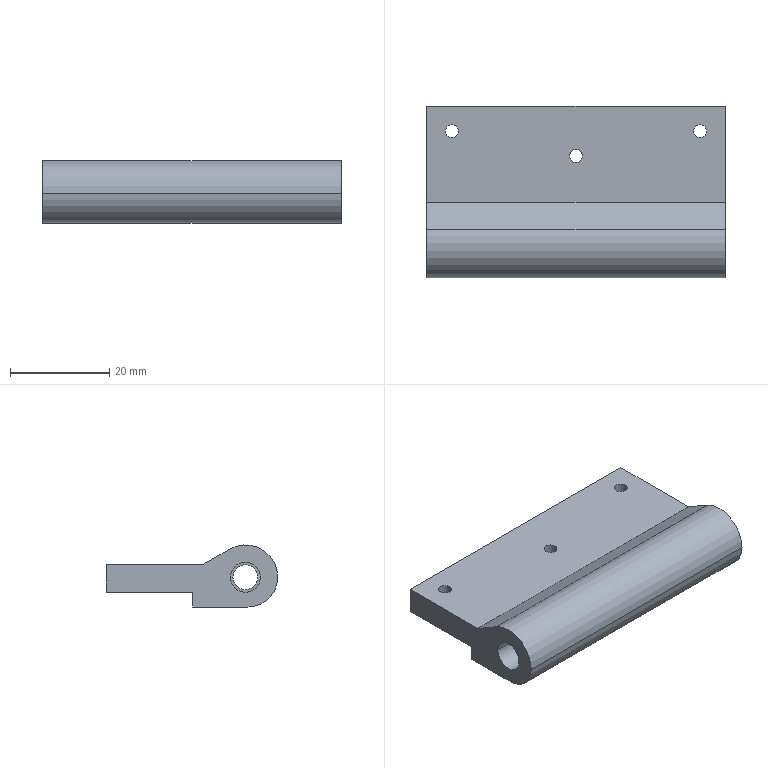NC program | NX | posted with a generic post | part box 60 x 34.5 x 12.5 mm
Whole program:
N10 G17 G21 G94 G90
(FACE_MILLING , TOOL : D63)
N12 T01 M6
N14 G54
N16 G17 G0 G90 X-97.5 Y20.5 B0. C0. S6500 M3
N18 G43 Z42.5 H1
N20 Z17.167
N22 G94 G1 Z14.167 F1250.
N24 X-66.
N26 X31.5
N28 Y-20.5
N30 X-66.
N32 X-97.5
N34 Z17.167
N36 G0 Z42.5
N38 Y20.5
N40 Z16.333
N42 G1 Z13.333
N44 X-66.
N46 X31.5
N48 Y-20.5
N50 X-66.
N52 X-97.5
N54 Z16.333
N56 G0 Z42.5
N58 Y20.5
N60 Z15.5
N62 G1 Z12.5
N64 X-66.
N66 X31.5
N68 Y-20.5
N70 X-66.
N72 X-97.5
N74 Z15.5
N76 G0 Z42.5
N78 M5
(FLOOR_WALL_2 , TOOL : D10)
N80 T10 M6
N82 G54
N84 G17 G0 G90 X-0.003 Y38. B0. C0. S9500 M3
N86 G43 Z42.5 H10
N88 Z14.525
N90 G94 G1 Z11.525 F2000.
N92 Y35.
N94 Y-35.
N96 X-4.786
N98 Y35.
N100 X-9.57
N102 Y-35.
N104 X-14.353
N106 Y35.
N108 Y38.
N110 Z14.525
N112 G0 Z42.5
N114 X-0.003
N116 Z13.55
N118 G1 Z10.55
N120 Y35.
N122 Y-35.
N124 X-4.786
N126 Y35.
N128 X-9.57
N130 Y-35.
N132 X-14.353
N134 Y35.
N136 Y38.
N138 Z13.55
N140 G0 Z42.5
N142 X-0.003
N144 Z12.575
N146 G1 Z9.575
N148 Y35.
N150 Y-35.
N152 X-4.786
N154 Y35.
N156 X-9.57
N158 Y-35.
N160 X-14.353
N162 Y35.
N164 Y38.15
N166 Z12.575
N168 G0 Z42.5
N170 X-0.003 Y38.
N172 Z11.6
N174 G1 Z8.6
N176 Y35.
N178 Y-35.
N180 X-4.786
N182 Y35.
N184 X-9.57
N186 Y-35.
N188 X-14.353
N190 Y35.
N192 Y38.15
N194 Z11.6
N196 G0 Z42.5
N198 M5
(FLOOR_WALL_1_COPY , TOOL : D10JING)
N200 T11 M6
N202 G54
N204 G17 G0 G90 X-0.001 Y38. B0. C0. S9500 M3
N206 G43 Z42.5 H11
N208 Z11.5
N210 G94 G1 Z8.5 F1250.
N212 Y35.
N214 Y-35.
N216 X-4.611
N218 Y35.
N220 X-9.22
N222 Y-35.
N224 X-13.83
N226 Y35.
N228 Y38.
N230 Z11.5
N232 G0 Z42.5
N234 X-14.33
N236 Z11.5
N238 G1 Z8.5
N240 Y35.
N242 Y-35.
N244 Y-38.
N246 Z11.5
N248 G0 Z42.5
N250 M5
(ZLEVEL_PROFILE_COPY_COPY_1_COPY_1_COPY_1_COPY , TOOL : D6R0.5)
N252 T05 M6
N254 G54
N256 G17 G0 G90 X-31.882 Y-30.701 B0. C0. S9500 M3
N258 G43 Z42.5 H5
N260 Z13.495
N262 G94 G1 Z12.495 F1000.
N264 X-31.26 Y-30.591
N266 G3 X-30.765 Y-30. R0.6
N268 G1 Y30. F3000.
N270 G2 X-25.543 Y31.205 R2.778
N272 X-25.235 Y30. R13.146
N274 G1 Y-30.
N276 G2 X-27.088 Y-32.519 R2.804
N278 G1 X-27.258 Y-32.565
N280 X-28.63 Y-32.57
N282 X-28.818 Y-32.522
N284 G2 X-30.765 Y-30. R2.757
N286 G1 X-30.818 Y-30.009 Z12.493
N288 X-30.871 Y-30.018 Z12.49
N290 X-30.774 Y-30.589
N292 G3 X-25.126 Y-30. R2.861
N294 G1 Y30.
N296 G3 X-25.681 Y31.678 R3.879
N298 X-30.874 Y30. R2.899
N300 G1 Y-30.
N302 X-30.871 Y-30.018
N304 X-30.914 Y-30.023 Z12.488
N306 X-30.955 Y-30.027 Z12.485
N308 X-30.958 Y-30.
N310 Y30.
N312 G2 X-29.003 Y32.909 R3.461
N314 X-25.407 Y31.324 R2.586
N316 X-25.042 Y30. R3.424
N318 G1 Y-30.
N320 G2 X-25.345 Y-31.221 R3.671
N322 G1 X-25.447 Y-31.452
N324 G2 X-29.917 Y-32.255 R2.739
N326 X-30.955 Y-30.027 R3.737
N328 G1 X-30.992 Y-30.03 Z12.483
N330 X-31.026 Y-30.033 Z12.48
N332 G3 X-30.491 Y-31.626 R3.549
N334 X-25.555 Y-31.898 R2.715
N336 X-24.971 Y-30. R5.44
N338 G1 Y30.
N340 G3 X-25.303 Y31.286 R3.708
N342 X-30.002 Y32.447 R2.738
N344 X-31.029 Y30. R4.971
N346 G1 Y-30.
N348 X-31.026 Y-30.033
N350 X-31.088 Y-30.038 Z12.475
N352 X-31.091 Y-30.
N354 Y30.
N356 G2 X-30.572 Y31.626 R3.637
N358 X-25.4 Y31.765 R2.709
N360 G1 X-25.253 Y31.333
N362 X-25.206 Y31.231
N364 G2 X-24.909 Y30. R3.255
N366 G1 Y-30.
N368 G2 X-25.55 Y-32.112 R6.321
N370 X-30.572 Y-31.626 R2.71
N372 X-31.088 Y-30.038 R3.636
N374 G1 X-31.147 Y-30.039 Z12.47
N376 G3 X-31.008 Y-30.736 R1.969
N378 G1 X-30.517 Y-31.971
N380 X-30.396 Y-32.317
N382 G3 X-25.886 Y-32.937 R2.789
N384 X-24.853 Y-30. R7.239
N386 G1 Y30.
N388 G3 X-25.316 Y31.728 R5.646
N390 G1 X-25.349 Y31.805
N392 X-25.462 Y32.136
N394 G3 X-29.186 Y33.485 R2.536
N396 X-30.792 Y31.28 R3.563
N398 X-31.147 Y30. R2.826
N400 G1 Y-30.008
N402 Y-30.039
N404 G2 X-31.634 Y-30.637 R0.6
N406 G1 X-32.258 Y-30.757
N408 Z13.47
N410 G0 X-25.591 Y34.555 Z13.465
N412 G1 Z12.465 F1000.
N414 X-25.986 Y34.041
N416 G3 X-25.953 Y33.27 R0.6
N418 G2 X-25.276 Y31.822 R2.673 F3000.
N420 X-24.801 Y30. R7.588
N422 G1 Y-30.
N424 G2 X-25.953 Y-33.27 R8.516
N426 G3 X-25.834 Y-34.032 R0.6
N428 G1 X-25.405 Y-34.407
N430 Z13.465
N432 G0 X-24.371 Y-34.116 Z13.46
N434 G1 Z12.46 F1000.
N436 X-25.044 Y-33.933
N438 G2 X-25.484 Y-33.3 R0.6
N440 G1 X-25.458 Y-33.008 F3000.
N442 X-24.945 Y-30.934
N444 X-24.857 Y-30.697
N446 X-24.828 Y-30.589
N448 X-24.753 Y-30.
N450 Y30.
N452 X-24.828 Y30.589
N454 X-24.857 Y30.717
N456 G2 X-25.482 Y33.3 R12.123
N458 G1 X-25.297 Z12.458
N460 X-25.298 Z12.455
N462 G3 X-24.885 Y30.934 R8.397
N464 G2 X-24.708 Y30. R3.901
N466 G1 Y-30.
N468 G2 X-24.885 Y-30.925 R3.578
N470 G3 X-25.305 Y-33.3 R8.261
N472 G1 X-25.207 Z12.453
N474 X-25.171 Z12.45
N476 G2 X-24.857 Y-31. R6.34
N478 G3 X-24.665 Y-30. R4.882
N480 G1 Y30.
N482 G3 X-24.844 Y30.934 R4.184
N484 G2 X-25.168 Y33.3 R6.488
N486 G1 X-25.104 Z12.447
N488 X-25.081 Z12.444
N490 G3 X-24.882 Y31.324 R6.216
N492 G2 X-24.614 Y30. R11.039
N494 G1 Y-30.
N496 X-24.641 Y-30.243
N498 X-25.036 Y-31.971
N500 X-25.083 Y-33.3
N502 X-24.993 Z12.44
N504 X-24.987 Z12.437
N506 X-24.96 Y-31.971
N508 X-24.584 Y-30.243
N510 X-24.562 Y-30.
N512 Y30.002
N514 G3 X-24.643 Y30.547 R1.863
N516 G2 X-24.986 Y33.3 R8.062
N518 G1 X-24.913 Z12.433
N520 X-24.878 Z12.429
N522 G3 X-24.572 Y30.462 R7.953
N524 G2 X-24.505 Y30.003 R1.62
N526 G1 Y-30.
N528 X-24.517 Y-30.243
N530 X-24.707 Y-31.045
N532 G3 X-24.878 Y-33.3 R7.252
N534 G1 X-24.832 Z12.424
N536 X-24.797 Z12.419
N538 G2 X-24.627 Y-30.934 R7.997
N540 G1 X-24.562 Y-30.746
N542 G3 X-24.439 Y-30.021 R2.207
N544 G1 Y30.018
N546 G3 X-24.563 Y30.749 R2.227
N548 G1 X-24.627 Y30.934
N550 G2 X-24.797 Y33.3 R7.995
N552 G1 X-24.755 Z12.413
N554 X-24.714 Z12.408
N556 G3 X-24.546 Y30.934 R8.119
N558 G1 X-24.514 Y30.842
N560 X-24.367 Y30.
N562 Y-30.
N564 X-24.514 Y-30.842
N566 X-24.546 Y-30.934
N568 G3 X-24.714 Y-33.3 R8.121
N570 G1 X-24.668 Z12.401
N572 X-24.623 Z12.395
N574 G2 X-24.528 Y-31.329 R7.767
N576 G1 X-24.292 Y-30.
N578 Y30.
N580 X-24.528 Y31.329
N582 G2 X-24.623 Y33.3 R7.765
N584 G1 X-24.572 Z12.388
N586 X-24.523 Z12.381
N588 G3 X-24.215 Y30. R16.402
N590 G1 Y-30.
N592 G3 X-24.523 Y-33.3 R16.402
N594 G1 X-24.466 Z12.373
N596 X-24.412 Z12.366
N598 G2 X-24.135 Y-30. R16.825
N600 G1 Y30.
N602 G2 X-24.412 Y33.3 R16.825
N604 G1 X-24.35 Z12.357
N606 X-24.292 Z12.349
N608 G3 X-24.053 Y30. R18.819
N610 G1 Y-30.
N612 G3 X-24.292 Y-33.3 R18.819
N614 G1 X-24.23 Z12.34
N616 X-24.166 Z12.331
N618 G2 X-23.969 Y-30. R18.207
N620 G1 Y30.
N622 G2 X-24.166 Y33.3 R18.207
N624 G1 X-24.126 Z12.321
N626 X-24.087 Z12.311
N628 G3 X-23.883 Y30. R17.398
N630 G1 Y-30.
N632 G3 X-24.087 Y-33.3 R17.398
N634 G1 X-24.041 Z12.3
N636 X-24.002 Z12.29
N638 G2 X-23.797 Y-30. R17.266
N640 G1 Y30.
N642 G2 X-24.002 Y33.3 R17.267
N644 G1 X-23.955 Z12.278
N646 X-23.912 Z12.267
N648 G3 X-23.709 Y30. R17.198
N650 G1 Y-30.
N652 G3 X-23.912 Y-33.3 R17.197
N654 G1 X-23.863 Z12.255
N656 X-23.816 Z12.243
N658 G2 X-23.621 Y-30. R18.12
N660 G1 Y30.
N662 G2 X-23.816 Y33.3 R18.121
N664 G1 X-23.766 Z12.23
N666 X-23.717 Z12.218
N668 G3 X-23.533 Y30. R19.742
N670 G1 Y-30.
N672 G3 X-23.717 Y-33.3 R19.742
N674 G1 X-23.663 Z12.204
N676 X-23.611 Z12.191
N678 G2 X-23.443 Y-30. R22.779
N680 G1 Y30.
N682 G2 X-23.611 Y33.3 R22.78
N684 G1 X-23.555 Z12.177
N686 X-23.5 Z12.163
N688 G3 X-23.354 Y30. R23.853
N690 G1 Y-30.
N692 G3 X-23.5 Y-33.3 R23.878
N694 G1 X-23.448 Z12.148
N696 X-23.412 Z12.133
N698 G2 X-23.265 Y-30. R22.34
N700 G1 Y30.
N702 G2 X-23.412 Y33.3 R22.341
N704 G1 X-23.356 Z12.118
N706 X-23.324 Z12.103
N708 G3 X-23.175 Y30. R21.933
N710 G1 Y-30.
N712 G3 X-23.324 Y-33.3 R21.932
N714 G1 X-23.27 Z12.087
N716 X-23.233 Z12.07
N718 G2 X-23.085 Y-30. R22.294
N720 G1 Y30.
N722 G2 X-23.233 Y33.3 R22.295
N724 G1 X-23.182 Z12.054
N726 X-23.138 Z12.037
N728 G3 X-22.996 Y30. R22.783
N730 G1 Y-30.
N732 G3 X-23.138 Y-33.3 R22.782
N734 G1 X-23.091 Z12.019
N736 X-23.045 Z12.002
N738 G2 X-22.907 Y-30. R23.686
N740 G1 Y30.
N742 G2 X-23.045 Y33.3 R23.687
N744 G1 X-22.996 Z11.984
N746 X-22.948 Z11.966
N748 G3 X-22.818 Y30. R25.767
N750 G1 Y-30.
N752 G3 X-22.948 Y-33.3 R25.766
N754 G1 X-22.897 Z11.947
N756 X-22.847 Z11.928
N758 G2 X-22.729 Y-30. R30.005
N760 G1 Y30.
N762 G2 X-22.847 Y33.3 R30.02
N764 G1 X-22.795 Z11.909
N766 X-22.755 Z11.889
N768 G3 X-22.64 Y30. R28.244
N770 G1 Y-30.
N772 G3 X-22.754 Y-33.3 R27.933
N774 G1 X-22.7 Z11.869
N776 X-22.668 Z11.849
N778 G2 X-22.552 Y-30. R27.65
N780 G1 Y30.
N782 G2 X-22.669 Y33.3 R28.528
N784 G1 X-22.612 Z11.828
N786 X-22.58 Z11.807
N788 G3 X-22.464 Y30. R29.201
N790 G1 Y-30.
N792 G3 X-22.579 Y-33.3 R27.826
N794 G1 X-22.527 Z11.786
N796 X-22.487 Z11.764
N798 G2 X-22.376 Y-30. R29.456
N800 G1 Y30.
N802 G2 X-22.489 Y33.3 R31.675
N804 G1 X-22.443 Z11.742
N806 X-22.4 Z11.72
N808 G3 X-22.289 Y30. R31.894
N810 G1 Y-30.
N812 G3 X-22.397 Y-33.3 R28.757
N814 G1 X-22.351 Z11.697
N816 X-22.306 Z11.675
N818 G2 X-22.203 Y-30. R29.795
N820 G1 Y30.
N822 G2 X-22.31 Y33.3 R34.069
N824 G1 X-22.263 Z11.651
N826 X-22.217 Z11.628
N828 G3 X-22.117 Y30. R37.521
N830 G1 Y-30.
N832 G3 X-22.213 Y-33.3 R32.275
N834 G1 X-22.164 Z11.604
N836 X-22.117 Z11.58
N838 G2 X-22.031 Y-30. R34.953
N840 G1 Y30.
N842 G2 X-22.122 Y33.3 R42.871
N844 G1 X-22.075 Z11.556
N846 X-22.032 Z11.531
N848 G3 X-21.946 Y30. R46.868
N850 G1 Y-30.
N852 G3 X-22.026 Y-33.3 R37.471
N854 G1 X-21.976 Z11.506
N856 X-21.935 Z11.482
N858 G2 X-21.861 Y-30. R39.395
N860 G1 Y30.
N862 G2 X-21.942 Y33.3 R53.283
N864 G1 X-21.894 Z11.457
N866 X-21.851 Z11.432
N868 G3 X-21.775 Y30. R61.807
N870 G1 Y-30.
N872 G3 X-21.844 Y-33.3 R41.544
N874 G1 X-21.796 Z11.407
N876 X-21.752 Y-33.299 Z11.382
N878 G2 X-21.689 Y-30. R43.507
N880 G1 Y30.
N882 G2 X-21.76 Y33.3 R74.582
N884 G1 X-21.715 Z11.357
N886 X-21.67 Y33.299 Z11.332
N888 G3 X-21.602 Y30. R89.703
N890 G1 Y-30.
N892 G3 X-21.662 Y-33.299 R44.801
N894 G1 X-21.616 Z11.307
N896 X-21.571 Z11.282
N898 G2 X-21.515 Y-30. R46.175
N900 G1 Y30.
N902 G2 X-21.581 Y33.299 R104.909
N904 G1 X-21.536 Z11.257
N906 X-21.491 Z11.232
N908 G3 X-21.429 Y30. R126.332
N910 G1 Y-30.
N912 G3 X-21.481 Y-33.299 R47.637
N914 G1 X-21.435 Z11.207
N916 X-21.39 Z11.182
N918 X-21.391 Y-33.008
N920 X-21.367 Y-30.589
N922 X-21.342 Y-30.
N924 Y30.
N926 X-21.401 Y33.299
N928 X-21.356 Z11.157
N930 X-21.312 Z11.132
N932 X-21.256 Y30.
N934 Y-30.
N936 X-21.281 Y-30.589
N938 X-21.3 Y-33.299
N940 X-21.254 Z11.107
N942 X-21.21 Z11.082
N944 X-21.194 Y-30.589
N946 X-21.169 Y-30.
N948 Y30.
N950 X-21.222 Y33.299
N952 X-21.177 Z11.057
N954 X-21.132 Z11.032
N956 X-21.129 Y32.663
N958 X-21.082 Y30.
N960 Y-30.
N962 X-21.091 Y-30.243
N964 X-21.12 Y-33.008
N966 X-21.119 Y-33.299
N968 X-21.073 Z11.007
N970 X-21.029 Z10.982
N972 X-21.004 Y-30.243
N974 X-20.996 Y-30.
N976 Y30.
N978 X-21.041 Y33.008
N980 X-21.043 Y33.299
N982 X-20.998 Z10.957
N984 X-20.953 Z10.932
N986 X-20.909 Y30.
N988 Y-30.
N990 X-20.939 Y-33.008
N992 X-20.938 Y-33.299
N994 X-20.893 Z10.907
N996 X-20.848 Z10.882
N998 X-20.823 Y-30.
N1000 Y30.
N1002 X-20.861 Y33.008
N1004 X-20.863 Y33.299
N1006 X-20.818 Z10.857
N1008 X-20.774 Z10.832
N1010 X-20.736 Y30.
N1012 Y-30.
N1014 X-20.758 Y-33.299
N1016 X-20.712 Z10.807
N1018 X-20.669 Z10.782
N1020 X-20.649 Y-30.
N1022 Y30.
N1024 X-20.684 Y33.299
N1026 X-20.639 Z10.757
N1028 X-20.596 Z10.732
N1030 X-20.563 Y30.
N1032 Y-30.
N1034 X-20.581 Y-33.299
N1036 X-20.535 Z10.707
N1038 X-20.493 Y-33.298 Z10.682
N1040 X-20.476 Y-30.
N1042 Y30.
N1044 X-20.507 Y33.298
N1046 X-20.463 Z10.657
N1048 X-20.419 Z10.632
N1050 X-20.39 Y30.243
N1052 Y30.
N1054 Y-30.
N1056 X-20.404 Y-33.298
N1058 X-20.36 Z10.607
N1060 X-20.317 Z10.582
N1062 X-20.303 Y-30.
N1064 Y30.
N1066 Y30.243
N1068 X-20.33 Y33.298
N1070 X-20.286 Z10.557
N1072 X-20.242 Z10.532
N1074 X-20.218 Y30.589
N1076 X-20.216 Y30.
N1078 Y-30.
N1080 X-20.23 Y-32.663
N1082 X-20.229 Y-33.298
N1084 X-20.185 Z10.507
N1086 X-20.142 Z10.482
N1088 Y-32.663
N1090 X-20.13 Y-30.
N1092 Y30.
N1094 X-20.154 Y33.298
N1096 X-20.109 Z10.457
N1098 X-20.065 Z10.432
N1100 X-20.043 Y30.
N1102 Y-30.
N1104 X-20.054 Y-33.008
N1106 Y-33.298
N1108 X-20.01 Z10.407
N1110 X-19.967 Z10.382
N1112 X-19.957 Y-30.
N1114 Y30.
N1116 X-19.971 Y32.663
N1118 X-19.977 Y33.297
N1120 X-19.933 Z10.357
N1122 X-19.889 Z10.332
N1124 X-19.886 Y33.008
N1126 X-19.87 Y30.243
N1128 Y30.
N1130 Y-30.
N1132 X-19.877 Y-30.589
N1134 X-19.879 Y-33.297
N1136 X-19.835 Z10.307
N1138 X-19.792 Z10.282
N1140 X-19.79 Y-30.589
N1142 X-19.783 Y-30.
N1144 Y30.
N1146 X-19.784 Y30.243
N1148 X-19.797 Y33.008
N1150 X-19.801 Y33.297
N1152 X-19.756 Z10.257
N1154 X-19.712 Z10.232
N1156 X-19.709 Y33.008
N1158 X-19.697 Y30.243
N1160 Y30.
N1162 Y-30.
N1164 X-19.704 Y-30.589
N1166 Y-33.297
N1168 X-19.66 Z10.207
N1170 X-19.617 Z10.182
N1172 X-19.616 Y-30.589
N1174 X-19.61 Y-30.
N1176 Y30.
N1178 X-19.611 Y30.243
N1180 X-19.624 Y33.297
N1182 X-19.58 Z10.157
N1184 X-19.536 Z10.132
N1186 X-19.524 Y30.
N1188 Y-30.
N1190 X-19.529 Y-33.297
N1192 X-19.485 Z10.107
N1194 X-19.442 Z10.082
N1196 X-19.44 Y-30.589
N1198 X-19.437 Y-30.
N1200 Y30.
N1202 X-19.448 Y33.297
N1204 X-19.403 Y33.296 Z10.057
N1206 X-19.36 Z10.032
N1208 X-19.35 Y30.
N1210 Y-30.
N1212 X-19.355 Y-33.296
N1214 X-19.31 Z10.007
N1216 X-19.268 Z9.982
N1218 X-19.264 Y-30.
N1220 Y30.
N1222 X-19.272 Y33.296
N1224 X-19.228 Z9.957
N1226 X-19.185 Z9.932
N1228 X-19.177 Y30.
N1230 Y-30.
N1232 X-19.181 Y-33.296
N1234 X-19.137 Z9.907
N1236 X-19.094 Y-33.295 Z9.882
N1238 X-19.091 Y-30.
N1240 Y30.
N1242 X-19.098 Y33.295
N1244 X-19.054 Z9.857
N1246 X-19.011 Z9.832
N1248 X-19.004 Y30.
N1250 Y-30.
N1252 X-19.007 Y-33.295
N1254 X-18.963 Z9.807
N1256 X-18.92 Z9.782
N1258 X-18.917 Y-30.
N1260 Y30.
N1262 X-18.924 Y33.295
N1264 X-18.88 Z9.757
N1266 X-18.837 Y33.294 Z9.732
N1268 X-18.831 Y30.
N1270 Y-30.
N1272 X-18.834 Y-33.294
N1274 X-18.79 Z9.707
N1276 X-18.747 Z9.682
N1278 X-18.744 Y-30.
N1280 Y30.
N1282 X-18.75 Y33.294
N1284 X-18.706 Z9.657
N1286 X-18.663 Z9.632
N1288 X-18.658 Y30.
N1290 Y-30.
N1292 X-18.66 Y-33.294
N1294 X-18.616 Y-33.293 Z9.607
N1296 X-18.573 Z9.582
N1298 X-18.571 Y-30.
N1300 Y30.
N1302 X-18.576 Y33.293
N1304 X-18.532 Z9.557
N1306 X-18.489 Z9.532
N1308 X-18.484 Y30.
N1310 Y-30.
N1312 X-18.487 Y-33.293
N1314 X-18.443 Z9.507
N1316 X-18.4 Z9.482
N1318 X-18.398 Y-30.
N1320 Y30.
N1322 X-18.402 Y33.292
N1324 X-18.358 Z9.457
N1326 X-18.315 Z9.432
N1328 X-18.311 Y30.
N1330 Y-30.
N1332 X-18.313 Y-33.292
N1334 X-18.269 Z9.407
N1336 X-18.226 Z9.382
N1338 X-18.225 Y-30.
N1340 Y30.
N1342 X-18.228 Y33.292
N1344 X-18.184 Z9.357
N1346 X-18.141 Y33.291 Z9.332
N1348 X-18.138 Y30.
N1350 Y-30.
N1352 X-18.14 Y-33.291
N1354 X-18.096 Z9.307
N1356 X-18.053 Z9.282
N1358 X-18.051 Y-30.
N1360 Y30.
N1362 X-18.054 Y33.291
N1364 X-18.01 Z9.257
N1366 X-17.967 Z9.232
N1368 X-17.965 Y30.
N1370 Y-30.
N1372 X-17.966 Y-33.291
N1374 X-17.922 Y-33.29 Z9.207
N1376 X-17.88 Z9.182
N1378 X-17.878 Y-30.
N1380 Y30.
N1382 X-17.88 Y33.29
N1384 X-17.836 Z9.157
N1386 X-17.794 Z9.132
N1388 X-17.792 Y30.
N1390 Y-30.
N1392 X-17.793 Y-33.29
N1394 X-17.749 Y-33.289 Z9.107
N1396 X-17.706 Z9.082
N1398 X-17.705 Y-30.
N1400 Y30.
N1402 X-17.707 Y33.289
N1404 X-17.663 Z9.057
N1406 X-17.62 Z9.032
N1408 X-17.618 Y30.
N1410 Y-30.
N1412 X-17.62 Y-33.289
N1414 X-17.576 Z9.007
N1416 X-17.533 Y-33.288 Z8.982
N1418 X-17.532 Y-30.
N1420 Y30.
N1422 X-17.534 Y33.288
N1424 X-17.49 Z8.957
N1426 X-17.447 Z8.932
N1428 X-17.445 Y30.
N1430 Y-30.
N1432 X-17.447 Y-33.288
N1434 X-17.403 Z8.907
N1436 X-17.36 Y-33.287 Z8.882
N1438 X-17.359 Y-30.
N1440 Y30.
N1442 X-17.361 Y33.287
N1444 X-17.317 Z8.857
N1446 X-17.274 Z8.832
N1448 X-17.272 Y30.
N1450 Y-30.
N1452 X-17.273 Y-33.287
N1454 X-17.229 Z8.807
N1456 X-17.187 Y-33.286 Z8.782
N1458 X-17.185 Y-30.
N1460 Y30.
N1462 X-17.187 Y33.286
N1464 X-17.143 Z8.757
N1466 X-17.101 Z8.732
N1468 X-17.099 Y30.
N1470 Y-30.
N1472 X-17.1 Y-33.286
N1474 X-17.056 Y-33.285 Z8.707
N1476 X-17.014 Z8.682
N1478 X-17.012 Y-30.
N1480 Y30.
N1482 X-17.014 Y33.285
N1484 X-16.97 Z8.657
N1486 X-16.928 Z8.632
N1488 X-16.926 Y30.
N1490 Y-30.
N1492 X-16.927 Y-33.285
N1494 X-16.883 Y-33.284 Z8.607
N1496 X-16.84 Z8.582
N1498 X-16.839 Y-30.
N1500 Y30.
N1502 X-16.841 Y33.284
N1504 X-16.797 Z8.557
N1506 X-16.754 Z8.532
N1508 X-16.752 Y30.
N1510 Y-30.
N1512 X-16.754 Y-33.284
N1514 G3 X-16.258 Y-33.875 R0.6
N1516 G1 X-15.621 Y-33.988
N1518 Z9.532
N1520 G0 Z42.5
N1522 X-30.187 Y-34.464
N1524 Z13.465
N1526 G1 Z12.465 F1000.
N1528 X-29.808 Y-34.049
N1530 G3 X-29.774 Y-33.279 R0.6
N1532 G1 X-30.512 Y-32.317 F3000.
N1534 G3 X-30.963 Y-31.04 R6.224
N1536 G2 X-31.199 Y-30.006 R2.384
N1538 G1 Y30.
N1540 G2 X-30.846 Y31.28 R2.833
N1542 X-30.345 Y32.613 R9.617
N1544 G1 X-29.769 Y33.281
N1546 G3 X-29.759 Y34.053 R0.6
N1548 G1 X-30.151 Y34.532
N1550 Z13.465
N1552 G0 X-30.224 Y33.301
N1554 G1 Z12.46 F1000.
N1556 G3 X-30.9 Y31.28 R19.06 F3000.
N1558 X-31.247 Y30. R2.996
N1560 G1 Y-30.001
N1562 G3 X-30.979 Y-31.125 R2.485
N1564 G1 X-30.9 Y-31.28
N1566 X-30.783 Y-31.626
N1568 X-30.418 Y-33.299
N1570 G2 X-30.777 Y-33.982 R0.6
N1572 G1 X-31.385 Y-34.232
N1574 Z13.46
N1576 G0 X-31.849 Y-34.025 Z13.455
N1578 G1 Z12.455 F1000.
N1580 X-31.204 Y-33.899
N1582 G3 X-30.718 Y-33.3 R0.6
N1584 G1 X-30.742 Y-31.971 F3000.
N1586 G3 X-31.066 Y-31.041 R5.052
N1588 G2 X-31.292 Y-30.007 R2.47
N1590 G1 Y30.008
N1592 G2 X-31.089 Y30.949 R2.274
N1594 G3 X-30.718 Y33.3 R4.456
N1596 G1 X-30.781 Z12.45
N1598 G2 X-31.139 Y30.945 R4.614
N1600 G3 X-31.335 Y30.007 R2.342
N1602 G1 Y-30.01
N1604 G3 X-31.121 Y-31.028 R2.52
N1606 G2 X-30.803 Y-31.971 R5.506
N1608 G1 X-30.781 Y-33.3
N1610 X-30.828 Z12.447
N1612 X-30.86 Z12.444
N1614 X-30.879 Y-31.971
N1616 G2 X-31.386 Y-30. R8.905
N1618 G1 Y30.002
N1620 G2 X-31.187 Y31. R2.598
N1622 G3 X-30.86 Y33.3 R4.64
N1624 G1 X-30.907 Z12.44
N1626 X-30.945 Z12.437
N1628 G2 X-31.286 Y30.934 R4.833
N1630 G1 X-31.438 Y30.
N1632 Y-30.
N1634 X-31.286 Y-30.934
N1636 G2 X-30.945 Y-33.3 R4.833
N1638 G1 X-30.996 Z12.433
N1640 X-31.043 Z12.429
N1642 X-31.056 Y-31.971
N1644 G2 X-31.495 Y-30. R8.333
N1646 G1 Y30.
N1648 G2 X-31.056 Y31.971 R8.334
N1650 G1 X-31.043 Y33.3
N1652 X-31.103 Z12.424
N1654 X-31.161 Z12.419
N1656 X-31.172 Y31.971
N1658 G3 X-31.561 Y30. R9.437
N1660 G1 Y-30.
N1662 G3 X-31.172 Y-31.971 R9.435
N1664 G1 X-31.161 Y-33.3
N1666 X-31.231 Z12.413
N1668 X-31.3 Z12.408
N1670 G3 X-31.633 Y-30. R15.358
N1672 G1 Y30.
N1674 G3 X-31.3 Y33.3 R15.358
N1676 G1 X-31.377 Z12.401
N1678 X-31.413 Z12.395
N1680 G2 X-31.708 Y30. R14.31
N1682 G1 Y-30.
N1684 G2 X-31.413 Y-33.3 R14.174
N1686 G1 X-31.482 Z12.388
N1688 X-31.495 Z12.381
N1690 G3 X-31.785 Y-30. R14.233
N1692 G1 Y30.
N1694 G3 X-31.495 Y33.3 R14.362
N1696 G1 X-31.566 Z12.373
N1698 X-31.587 Z12.366
N1700 G2 X-31.865 Y30. R14.451
N1702 G1 Y-30.
N1704 G2 X-31.587 Y-33.3 R14.451
N1706 G1 X-31.649 Z12.357
N1708 X-31.687 Z12.349
N1710 G3 X-31.947 Y-30. R14.37
N1712 G1 Y30.
N1714 G3 X-31.687 Y33.3 R14.789
N1716 G1 X-31.738 Z12.34
N1718 X-31.785 Z12.331
N1720 G2 X-32.031 Y30. R15.079
N1722 G1 Y-30.
N1724 G2 X-31.785 Y-33.3 R15.079
N1726 G1 X-31.836 Z12.321
N1728 X-31.886 Z12.311
N1730 G3 X-32.117 Y-30. R16.576
N1732 G1 Y30.
N1734 G3 X-31.886 Y33.3 R16.576
N1736 G1 X-31.94 Z12.3
N1738 X-31.994 Z12.29
N1740 G2 X-32.203 Y30. R19.13
N1742 G1 Y-30.
N1744 G2 X-31.994 Y-33.3 R19.13
N1746 G1 X-32.052 Z12.278
N1748 X-32.106 Z12.267
N1750 G3 X-32.291 Y-30. R21.923
N1752 G1 Y30.
N1754 G3 X-32.106 Y33.3 R21.923
N1756 G1 X-32.164 Z12.255
N1758 X-32.219 Z12.243
N1760 G2 X-32.379 Y30. R22.455
N1762 G1 Y-30.
N1764 G2 X-32.219 Y-33.3 R22.455
N1766 G1 X-32.262 Z12.23
N1768 X-32.304 Z12.218
N1770 G3 X-32.467 Y-30. R20.803
N1772 G1 Y30.
N1774 G3 X-32.304 Y33.3 R20.804
N1776 G1 X-32.347 Z12.204
N1778 X-32.39 Z12.191
N1780 G2 X-32.557 Y30. R20.092
N1782 G1 Y-30.
N1784 G2 X-32.39 Y-33.3 R20.091
N1786 G1 X-32.435 Z12.177
N1788 X-32.479 Z12.163
N1790 G3 X-32.646 Y-30. R20.179
N1792 G1 Y30.
N1794 G3 X-32.479 Y33.3 R20.18
N1796 G1 X-32.527 Z12.148
N1798 X-32.574 Z12.133
N1800 G2 X-32.735 Y30. R21.108
N1802 G1 Y-30.
N1804 G2 X-32.574 Y-33.3 R21.107
N1806 G1 X-32.624 Z12.118
N1808 X-32.672 Z12.103
N1810 G3 X-32.825 Y-30. R22.308
N1812 G1 Y30.
N1814 G3 X-32.672 Y33.3 R22.308
N1816 G1 X-32.724 Z12.087
N1818 X-32.775 Z12.07
N1820 G2 X-32.915 Y30. R25.569
N1822 G1 Y-30.
N1824 G2 X-32.775 Y-33.3 R25.477
N1826 G1 X-32.829 Z12.054
N1828 X-32.883 Z12.037
N1830 G3 X-33.004 Y-30. R30.797
N1832 G1 Y30.
N1834 G3 X-32.883 Y33.3 R30.798
N1836 G1 X-32.929 Z12.019
N1838 X-32.974 Z12.002
N1840 G2 X-33.093 Y30. R28.017
N1842 G1 Y-30.
N1844 G2 X-32.974 Y-33.3 R28.016
N1846 G1 X-33.02 Z11.984
N1848 X-33.06 Z11.966
N1850 G3 X-33.182 Y-30. R27.428
N1852 G1 Y30.
N1854 G3 X-33.06 Y33.3 R27.429
N1856 G1 X-33.105 Z11.947
N1858 X-33.147 Z11.928
N1860 G2 X-33.271 Y30. R25.785
N1862 G1 Y-30.
N1864 G2 X-33.147 Y-33.3 R25.784
N1866 G1 X-33.192 Z11.909
N1868 X-33.236 Z11.889
N1870 G3 X-33.36 Y-30. R25.865
N1872 G1 Y30.
N1874 G3 X-33.236 Y33.3 R25.866
N1876 G1 X-33.282 Z11.869
N1878 X-33.328 Z11.849
N1880 G2 X-33.448 Y30. R27.049
N1882 G1 Y-30.
N1884 G2 X-33.328 Y-33.3 R27.048
N1886 G1 X-33.376 Z11.828
N1888 X-33.423 Z11.807
N1890 G3 X-33.536 Y-30. R29.178
N1892 G1 Y30.
N1894 G3 X-33.423 Y33.3 R29.179
N1896 G1 X-33.472 Z11.786
N1898 X-33.52 Z11.764
N1900 G2 X-33.624 Y30. R33.369
N1902 G1 Y-30.
N1904 G2 X-33.52 Y-33.3 R33.368
N1906 G1 X-33.571 Z11.742
N1908 X-33.618 Z11.72
N1910 G3 X-33.711 Y-30. R35.37
N1912 G1 Y30.
N1914 G3 X-33.618 Y33.3 R35.372
N1916 G1 X-33.661 Z11.697
N1918 X-33.701 Z11.675
N1920 G2 X-33.797 Y30. R34.132
N1922 G1 Y-30.
N1924 G2 X-33.701 Y-33.3 R34.131
N1926 G1 X-33.746 Z11.651
N1928 X-33.786 Z11.628
N1930 G3 X-33.883 Y-30. R32.693
N1932 G1 Y30.
N1934 G3 X-33.786 Y33.3 R32.694
N1936 G1 X-33.828 Z11.604
N1938 X-33.869 Z11.58
N1940 G2 X-33.969 Y30. R31.613
N1942 G1 Y-30.
N1944 G2 X-33.869 Y-33.3 R31.612
N1946 G1 X-33.912 Z11.556
N1948 X-33.954 Z11.531
N1950 G3 X-34.053 Y-30. R31.828
N1952 G1 Y30.
N1954 G3 X-33.954 Y33.3 R31.829
N1956 G1 X-33.997 Z11.506
N1958 X-34.039 Z11.482
N1960 G2 X-34.136 Y30. R33.378
N1962 G1 Y-30.
N1964 G2 X-34.039 Y-33.3 R33.377
N1966 G1 X-34.082 Z11.457
N1968 X-34.125 Z11.432
N1970 G3 X-34.216 Y-30. R35.962
N1972 G1 Y30.
N1974 G3 X-34.125 Y33.3 R35.964
N1976 G1 X-34.169 Z11.407
N1978 X-34.211 Z11.382
N1980 G2 X-34.294 Y30. R40.823
N1982 G1 Y-30.
N1984 G2 X-34.211 Y-33.3 R40.822
N1986 G1 X-34.254 Z11.357
N1988 X-34.296 Z11.332
N1990 G3 X-34.371 Y-30. R43.574
N1992 G1 Y30.
N1994 G3 X-34.296 Y33.3 R44.659
N1996 G1 X-34.331 Z11.307
N1998 X-34.366 Z11.282
N2000 G2 X-34.445 Y30. R40.598
N2002 G1 Y-30.
N2004 G2 X-34.366 Y-33.3 R40.597
N2006 G1 X-34.402 Z11.257
N2008 X-34.435 Z11.232
N2010 G3 X-34.517 Y-30. R38.825
N2012 G1 Y30.
N2014 G3 X-34.435 Y33.3 R38.827
N2016 G1 X-34.47 Z11.207
N2018 X-34.504 Z11.182
N2020 G2 X-34.588 Y30. R37.3
N2022 G1 Y-30.
N2024 G2 X-34.504 Y-33.3 R37.393
N2026 G1 X-34.538 Z11.157
N2028 X-34.572 Z11.132
N2030 G3 X-34.656 Y-30. R37.015
N2032 G1 Y30.
N2034 G3 X-34.572 Y33.3 R36.932
N2036 G1 X-34.606 Z11.107
N2038 X-34.64 Z11.082
N2040 G2 X-34.723 Y30. R37.734
N2042 G1 Y-30.
N2044 G2 X-34.64 Y-33.3 R37.732
N2046 G1 X-34.674 Z11.057
N2048 X-34.708 Z11.032
N2050 G3 X-34.789 Y-30. R39.621
N2052 G1 Y30.
N2054 G3 X-34.708 Y33.3 R39.622
N2056 G1 X-34.742 Z11.007
N2058 X-34.776 Z10.982
N2060 G2 X-34.852 Y30. R43.779
N2062 G1 Y-30.
N2064 G2 X-34.776 Y-33.3 R43.828
N2066 G1 X-34.81 Z10.957
N2068 X-34.841 Z10.932
N2070 G3 X-34.915 Y-30. R42.858
N2072 G1 Y30.
N2074 G3 X-34.841 Y33.3 R42.859
N2076 G1 X-34.878 Z10.907
N2078 X-34.905 Z10.882
N2080 G2 X-34.975 Y30. R47.063
N2082 G1 Y-30.
N2084 G2 X-34.905 Y-33.3 R47.062
N2086 G1 X-34.939 Z10.857
N2088 X-34.968 Z10.832
N2090 G3 X-35.035 Y-30. R50.531
N2092 G1 Y30.
N2094 G3 X-34.968 Y33.3 R50.533
N2096 G1 X-34.996 Z10.807
N2098 X-35.023 Z10.782
N2100 G2 X-35.093 Y30. R45.547
N2102 G1 Y-30.
N2104 G2 X-35.023 Y-33.3 R45.545
N2106 G1 X-35.051 Z10.757
N2108 X-35.078 Z10.732
N2110 G3 X-35.15 Y-30. R43.572
N2112 G1 Y30.
N2114 G3 X-35.078 Y33.3 R43.588
N2116 G1 X-35.105 Z10.707
N2118 X-35.132 Z10.682
N2120 G2 X-35.206 Y30. R42.402
N2122 G1 Y-30.
N2124 G2 X-35.132 Y-33.3 R42.401
N2126 G1 X-35.159 Z10.657
N2128 X-35.186 Z10.632
N2130 G3 X-35.26 Y-30. R42.103
N2132 G1 Y30.
N2134 G3 X-35.186 Y33.3 R42.105
N2136 G1 X-35.214 Z10.607
N2138 X-35.24 Z10.582
N2140 G2 X-35.313 Y30. R42.734
N2142 G1 Y-30.
N2144 G2 X-35.24 Y-33.3 R42.733
N2146 G1 X-35.268 Z10.557
N2148 X-35.294 Z10.532
N2150 G3 X-35.366 Y-30. R44.356
N2152 G1 Y30.
N2154 G3 X-35.294 Y33.3 R44.358
N2156 G1 X-35.322 Z10.507
N2158 X-35.348 Z10.482
N2160 G2 X-35.417 Y30. R47.178
N2162 G1 Y-30.
N2164 G2 X-35.348 Y-33.3 R47.176
N2166 G1 X-35.377 Z10.457
N2168 X-35.402 Z10.432
N2170 G3 X-35.467 Y-30. R51.617
N2172 G1 Y30.
N2174 G3 X-35.402 Y33.3 R51.618
N2176 G1 X-35.431 Z10.407
N2178 X-35.457 Z10.382
N2180 G2 X-35.516 Y30. R59.563
N2182 G1 Y-30.
N2184 G2 X-35.457 Y-33.3 R59.562
N2186 G1 X-35.481 Z10.357
N2188 X-35.507 Z10.332
N2190 G3 X-35.564 Y-30. R55.364
N2192 G1 Y30.
N2194 G3 X-35.507 Y33.3 R55.366
N2196 G1 X-35.529 Z10.307
N2198 X-35.55 Z10.282
N2200 G2 X-35.612 Y30. R51.039
N2202 G1 Y-30.
N2204 G2 X-35.55 Y-33.3 R51.037
N2206 G1 X-35.573 Z10.257
N2208 X-35.594 Z10.232
N2210 G3 X-35.658 Y-30. R48.196
N2212 G1 Y30.
N2214 G3 X-35.594 Y33.3 R48.197
N2216 G1 X-35.617 Z10.207
N2218 X-35.638 Z10.182
N2220 G2 X-35.703 Y30. R46.849
N2222 G1 Y-30.
N2224 G2 X-35.638 Y-33.3 R46.848
N2226 G1 X-35.66 Z10.157
N2228 X-35.681 Z10.132
N2230 G3 X-35.748 Y-30. R46.194
N2232 G1 Y30.
N2234 G3 X-35.681 Y33.3 R46.196
N2236 G1 X-35.704 Z10.107
N2238 X-35.725 Z10.082
N2240 G2 X-35.792 Y30. R46.425
N2242 G1 Y-30.
N2244 G2 X-35.725 Y-33.3 R46.424
N2246 G1 X-35.747 Z10.057
N2248 X-35.769 Z10.032
N2250 G3 X-35.835 Y-30. R47.358
N2252 G1 Y30.
N2254 G3 X-35.769 Y33.3 R47.367
N2256 G1 X-35.791 Z10.007
N2258 X-35.812 Z9.982
N2260 G2 X-35.877 Y30. R49.024
N2262 G1 Y-30.
N2264 G2 X-35.812 Y-33.3 R49.022
N2266 G1 X-35.834 Z9.957
N2268 X-35.855 Z9.932
N2270 G3 X-35.918 Y-30. R51.204
N2272 G1 Y30.
N2274 G3 X-35.855 Y33.3 R51.206
N2276 G1 X-35.878 Z9.907
N2278 X-35.898 Z9.882
N2280 G2 X-35.958 Y30. R54.419
N2282 G1 Y-30.
N2284 G2 X-35.898 Y-33.3 R54.414
N2286 G1 X-35.922 Z9.857
N2288 X-35.941 Z9.832
N2290 G3 X-35.998 Y-30. R56.485
N2292 G1 Y30.
N2294 G3 X-35.941 Y33.3 R56.487
N2296 G1 X-35.964 Z9.807
N2298 X-35.984 Z9.782
N2300 G2 X-36.037 Y30. R67.786
N2302 G1 Y-30.
N2304 G2 X-35.984 Y-33.3 R67.784
N2306 G1 X-36.003 Z9.757
N2308 X-36.022 Z9.732
N2310 G3 X-36.076 Y-30. R60.536
N2312 G1 Y30.
N2314 G3 X-36.022 Y33.3 R60.538
N2316 G1 X-36.04 Z9.707
N2318 X-36.057 Z9.682
N2320 G2 X-36.113 Y30. R56.448
N2322 G1 Y-30.
N2324 G2 X-36.057 Y-33.3 R56.446
N2326 G1 X-36.075 Z9.657
N2328 X-36.092 Z9.632
N2330 G3 X-36.15 Y-30. R53.784
N2332 G1 Y30.
N2334 G3 X-36.092 Y33.3 R53.668
N2336 G1 X-36.109 Z9.607
N2338 X-36.126 Z9.582
N2340 G2 X-36.186 Y30. R52.203
N2342 G1 Y-30.
N2344 G2 X-36.126 Y-33.3 R52.201
N2346 G1 X-36.144 Z9.557
N2348 X-36.161 Z9.532
N2350 G3 X-36.222 Y-30. R51.175
N2352 G1 Y30.
N2354 G3 X-36.161 Y33.3 R51.038
N2356 G1 X-36.179 Z9.507
N2358 X-36.196 Z9.482
N2360 G2 X-36.257 Y30. R50.856
N2362 G1 Y-30.
N2364 G2 X-36.196 Y-33.3 R50.854
N2366 G1 X-36.213 Z9.457
N2368 X-36.23 Z9.432
N2370 G3 X-36.291 Y-30. R51.3
N2372 G1 Y30.
N2374 G3 X-36.23 Y33.3 R51.302
N2376 G1 X-36.248 Z9.407
N2378 X-36.265 Z9.382
N2380 G2 X-36.325 Y30. R52.548
N2382 G1 Y-30.
N2384 G2 X-36.265 Y-33.3 R52.546
N2386 G1 X-36.283 Z9.357
N2388 X-36.3 Z9.332
N2390 G3 X-36.358 Y-30. R54.696
N2392 G1 Y30.
N2394 G3 X-36.3 Y33.3 R54.596
N2396 G1 X-36.317 Z9.307
N2398 X-36.334 Z9.282
N2400 G2 X-36.39 Y30. R57.584
N2402 G1 Y-30.
N2404 G2 X-36.334 Y-33.3 R57.582
N2406 G1 X-36.369 Z9.232
N2408 G3 X-36.422 Y-30. R61.51
N2410 G1 Y30.
N2412 G3 X-36.369 Y33.3 R61.512
N2414 G1 X-36.403 Z9.182
N2416 G2 X-36.453 Y30. R69.425
N2418 G1 Y-30.
N2420 G2 X-36.403 Y-33.3 R69.423
N2422 G1 X-36.436 Z9.132
N2424 G3 X-36.484 Y-30. R67.148
N2426 G1 Y30.
N2428 G3 X-36.436 Y33.3 R67.151
N2430 G1 X-36.463 Z9.082
N2432 G2 X-36.514 Y30. R63.159
N2434 G1 Y-30.
N2436 G2 X-36.463 Y-33.3 R63.156
N2438 G1 X-36.49 Z9.032
N2440 G3 X-36.543 Y-30. R60.26
N2442 G1 Y30.
N2444 G3 X-36.49 Y33.3 R60.262
N2446 G1 X-36.518 Z8.982
N2448 G2 X-36.572 Y30. R57.347
N2450 G1 Y-30.
N2452 G2 X-36.518 Y-33.3 R57.502
N2454 G1 X-36.545 Z8.932
N2456 G3 X-36.601 Y-30. R55.602
N2458 G1 Y30.
N2460 G3 X-36.545 Y33.3 R55.604
N2462 G1 X-36.572 Z8.882
N2464 G2 X-36.629 Y30. R54.669
N2466 G1 Y-30.
N2468 G2 X-36.572 Y-33.3 R54.668
N2470 G1 X-36.599 Z8.832
N2472 G3 X-36.656 Y-30. R54.393
N2474 G1 Y30.
N2476 G3 X-36.599 Y33.3 R54.394
N2478 G1 X-36.626 Z8.782
N2480 G2 X-36.683 Y30. R54.699
N2482 G1 Y-30.
N2484 G2 X-36.626 Y-33.3 R54.697
N2486 G1 X-36.653 Z8.732
N2488 G3 X-36.709 Y-30. R55.749
N2490 G1 Y30.
N2492 G3 X-36.653 Y33.3 R55.634
N2494 G1 X-36.68 Z8.682
N2496 G2 X-36.735 Y30. R58.158
N2498 G1 Y-30.
N2500 G2 X-36.68 Y-33.3 R58.156
N2502 G1 X-36.707 Z8.632
N2504 G3 X-36.76 Y-30. R59.352
N2506 G1 Y30.
N2508 G3 X-36.707 Y33.3 R59.354
N2510 G1 X-36.734 Z8.582
N2512 G2 X-36.785 Y30. R61.24
N2514 G1 Y-30.
N2516 G2 X-36.734 Y-33.3 R61.238
N2518 G1 X-36.761 Z8.532
N2520 G3 X-36.809 Y-30. R64.264
N2522 G1 Y30.
N2524 G3 X-36.761 Y33.3 R64.266
N2526 G1 X-36.786 Z8.482
N2528 G2 X-36.833 Y30. R64.425
N2530 G1 Y-30.
N2532 G2 X-36.786 Y-33.3 R64.423
N2534 G1 X-36.807 Z8.432
N2536 G3 X-36.856 Y-30. R64.571
N2538 G1 Y30.
N2540 G3 X-36.807 Y33.3 R64.573
N2542 G1 X-36.82 Z8.407
N2544 X-36.829 Z8.382
N2546 G2 X-36.879 Y30. R65.512
N2548 G1 Y-30.
N2550 G2 X-36.829 Y-33.3 R65.51
N2552 G1 X-36.841 Z8.357
N2554 X-36.85 Z8.332
N2556 G3 X-36.901 Y-30. R64.054
N2558 G1 Y30.
N2560 G3 X-36.85 Y33.3 R64.056
N2562 G1 X-36.871 Z8.282
N2564 G2 X-36.923 Y30. R59.858
N2566 G1 Y-30.
N2568 G2 X-36.871 Y-33.3 R59.856
N2570 G1 X-36.891 Z8.232
N2572 G3 X-36.945 Y-30. R58.283
N2574 G1 Y30.
N2576 G3 X-36.891 Y33.3 R58.285
N2578 G1 X-36.912 Z8.182
N2580 G2 X-36.966 Y30. R57.132
N2582 G1 Y-30.
N2584 G2 X-36.912 Y-33.3 R57.13
N2586 G1 X-36.932 Z8.132
N2588 G3 X-36.986 Y-30. R56.899
N2590 G1 Y30.
N2592 G3 X-36.932 Y33.3 R56.901
N2594 G1 X-36.952 Z8.082
N2596 G2 X-37.006 Y30. R57.165
N2598 G1 Y-30.
N2600 G2 X-36.952 Y-33.3 R57.164
N2602 G1 X-36.973 Z8.032
N2604 G3 X-37.026 Y-30. R58.437
N2606 G1 Y30.
N2608 G3 X-36.973 Y33.3 R58.439
N2610 G1 X-36.993 Z7.982
N2612 G2 X-37.045 Y30. R60.313
N2614 G1 Y-30.
N2616 G2 X-36.993 Y-33.3 R60.311
N2618 G1 X-37.013 Z7.932
N2620 G3 X-37.064 Y-30. R64.26
N2622 G1 Y30.
N2624 G3 X-37.013 Y33.3 R64.262
N2626 G1 X-37.034 Z7.882
N2628 G2 X-37.082 Y30. R66.358
N2630 G1 Y-30.
N2632 G2 X-37.034 Y-33.3 R66.356
N2634 G1 X-37.044 Z7.857
N2636 X-37.051 Z7.832
N2638 G3 X-37.1 Y-30. R67.5
N2640 G1 Y30.
N2642 G3 X-37.051 Y33.3 R67.501
N2644 G1 X-37.063 Z7.807
N2646 X-37.068 Z7.782
N2648 G2 X-37.117 Y30. R69.313
N2650 G1 Y-30.
N2652 G2 X-37.068 Y-33.3 R69.312
N2654 G1 X-37.079 Z7.757
N2656 X-37.085 Z7.732
N2658 G3 X-37.134 Y-30. R71.662
N2660 G1 Y30.
N2662 G3 X-37.085 Y33.3 R72.291
N2664 G1 X-37.096 Z7.707
N2666 X-37.102 Z7.682
N2668 G2 X-37.151 Y30. R72.21
N2670 G1 Y-30.
N2672 G2 X-37.102 Y-33.3 R72.209
N2674 G1 X-37.112 Z7.657
N2676 X-37.119 Z7.632
N2678 G3 X-37.167 Y-30. R66.635
N2680 G1 Y30.
N2682 G3 X-37.119 Y33.3 R66.637
N2684 G1 X-37.133 Z7.582
N2686 G2 X-37.183 Y30. R63.557
N2688 G1 Y-30.
N2690 G2 X-37.133 Y-33.3 R63.555
N2692 G1 X-37.148 Z7.532
N2694 G3 X-37.198 Y-30. R61.455
N2696 G1 Y30.
N2698 G3 X-37.148 Y33.3 R61.458
N2700 G1 X-37.162 Z7.482
N2702 G2 X-37.213 Y30. R60.191
N2704 G1 Y-30.
N2706 G2 X-37.162 Y-33.3 R60.189
N2708 G1 X-37.176 Z7.432
N2710 G3 X-37.228 Y-30. R59.136
N2712 G1 Y30.
N2714 G3 X-37.176 Y33.3 R59.138
N2716 G1 X-37.19 Z7.382
N2718 G2 X-37.242 Y30. R59.112
N2720 G1 Y-30.
N2722 G2 X-37.19 Y-33.3 R59.11
N2724 G1 X-37.204 Z7.332
N2726 G3 X-37.256 Y-30. R58.611
N2728 G1 Y30.
N2730 G3 X-37.204 Y33.3 R58.407
N2732 G1 X-37.218 Z7.282
N2734 G2 X-37.22 Y31.626 R365.838
N2736 G1 X-37.246 Y30.589
N2738 X-37.253 Y30.243
N2740 X-37.269 Y30.
N2742 Y-30.
N2744 X-37.253 Y-30.243
N2746 X-37.246 Y-30.589
N2748 G2 X-37.218 Y-33.3 R64.889
N2750 G1 X-37.232 Z7.232
N2752 G3 X-37.26 Y-30.589 R64.89
N2754 G1 X-37.266 Y-30.243
N2756 X-37.282 Y-30.
N2758 Y30.
N2760 X-37.266 Y30.243
N2762 X-37.26 Y30.589
N2764 X-37.234 Y31.626
N2766 G3 X-37.232 Y33.3 R365.863
N2768 G1 X-37.247 Z7.182
N2770 G2 X-37.275 Y30.589 R64.894
N2772 X-37.295 Y30. R5.047
N2774 G1 Y-30.
N2776 G2 X-37.275 Y-30.589 R5.047
N2778 X-37.247 Y-33.3 R64.891
N2780 G1 X-37.261 Z7.132
N2782 G3 X-37.289 Y-30.589 R65.046
N2784 X-37.307 Y-30. R4.727
N2786 G1 Y30.
N2788 G3 X-37.289 Y30.589 R4.727
N2790 X-37.261 Y33.3 R65.049
N2792 G1 X-37.275 Z7.082
N2794 G2 X-37.303 Y30.589 R64.99
N2796 X-37.319 Y30. R4.558
N2798 G1 Y-30.
N2800 G2 X-37.303 Y-30.589 R4.558
N2802 X-37.275 Y-33.3 R65.138
N2804 G1 X-37.277 Z7.057
N2806 X-37.285 Z7.032
N2808 G3 X-37.316 Y-30.589 R58.501
N2810 X-37.33 Y-30. R4.688
N2812 G1 Y30.
N2814 G3 X-37.316 Y30.589 R4.699
N2816 X-37.285 Y33.3 R58.081
N2818 G1 X-37.294 Z6.982
N2820 G2 X-37.325 Y30.589 R60.645
N2822 X-37.341 Y30. R6.336
N2824 G1 Y-30.
N2826 G2 X-37.294 Y-33.3 R72.068
N2828 G1 X-37.303 Z6.932
N2830 G3 X-37.352 Y-30. R69.704
N2832 G1 Y30.
N2834 G3 X-37.304 Y33.3 R68.339
N2836 G1 X-37.313 Z6.882
N2838 G2 X-37.362 Y30. R66.313
N2840 G1 Y-30.
N2842 G2 X-37.312 Y-33.3 R68.345
N2844 G1 X-37.321 Z6.832
N2846 G3 X-37.372 Y-30. R69.519
N2848 G1 Y30.
N2850 G3 X-37.322 Y33.3 R64.58
N2852 G1 X-37.331 Z6.795
N2854 X-37.336 Z6.758
N2856 G2 X-37.386 Y30. R62.838
N2858 G1 Y-30.
N2860 G2 X-37.335 Y-33.3 R68.098
N2862 G1 X-37.345 Z6.708
N2864 X-37.352 Z6.659
N2866 G3 X-37.403 Y-30. R66.832
N2868 G1 Y30.
N2870 G3 X-37.354 Y33.3 R61.392
N2872 G1 X-37.363 Z6.61
N2874 X-37.371 Z6.56
N2876 G2 X-37.419 Y30. R62.461
N2878 G1 Y-30.
N2880 G2 X-37.368 Y-33.3 R72.195
N2882 G1 X-37.378 Z6.511
N2884 X-37.384 Z6.461
N2886 G3 X-37.434 Y-30. R80.226
N2888 G1 Y30.
N2890 G3 X-37.388 Y33.3 R68.805
N2892 G1 X-37.397 Z6.412
N2894 X-37.404 Z6.362
N2896 G2 X-37.447 Y30. R76.905
N2898 G1 Y-30.
N2900 G2 X-37.4 Y-33.3 R91.835
N2902 G1 X-37.407 Y-33.301 Z6.313
N2904 X-37.416 Z6.263
N2906 G3 X-37.458 Y-30. R109.981
N2908 G1 Y30.
N2910 G3 X-37.421 Y33.3 R82.53
N2912 G1 X-37.428 Z6.213
N2914 X-37.434 Z6.163
N2916 G2 X-37.468 Y30. R87.939
N2918 G1 Y-30.
N2920 G2 X-37.429 Y-33.301 R134.259
N2922 G1 X-37.436 Y-33.302 Z6.114
N2924 X-37.441 Z6.064
N2926 G3 X-37.477 Y-30. R177.358
N2928 G1 Y30.
N2930 G3 X-37.447 Y33.3 R97.759
N2932 G1 X-37.454 Z6.014
N2934 X-37.46 Z5.964
N2936 Y31.626
N2938 X-37.463 Y31.28
N2940 X-37.473 Y30.243
N2942 X-37.485 Y30.
N2944 Y-30.
N2946 X-37.475 Y-30.243
N2948 X-37.452 Y-33.303
N2950 X-37.458 Z5.914
N2952 X-37.463 Z5.864
N2954 X-37.482 Y-30.243
N2956 X-37.491 Y-30.
N2958 Y30.
N2960 G3 X-37.482 Y30.589 R5.35
N2962 G1 X-37.473 Y30.934
N2964 X-37.469 Y33.3
N2966 X-37.477 Z5.773
N2968 X-37.48 Y30.934
N2970 X-37.486 Y30.589
N2972 G2 X-37.495 Y30. R6.135
N2974 G1 Y-30.
N2976 X-37.487 Y-30.243
N2978 X-37.473 Y-33.302
N2980 X-37.483 Y-33.301 Z5.682
N2982 X-37.498 Y-29.536
N2984 Y29.536
N2986 X-37.496 Y29.546
N2988 X-37.486 Y33.008
N2990 X-37.485 Y33.3
N2992 X-37.494 Z5.591
N2994 X-37.497 Y29.546
N2996 X-37.499 Y29.535
N2998 Y-29.535
N3000 X-37.493 Y-33.301
N3002 X-37.496 Y-33.302 Z5.5
N3004 X-37.5 Y-29.535
N3006 Y29.535
N3008 X-37.497 Y29.546
N3010 X-37.499 Y33.008
N3012 X-37.496 Y33.302
N3014 G3 X-37.987 Y33.898 R0.6
N3016 G1 X-38.635 Y34.018
N3018 Z6.5
N3020 G0 Z42.5
N3022 M5
(ZLEVEL_PROFILE_1_COPY_1_COPY_COPY_COPY_1_COPY_COPY_COPY_COPY_COPY , TOOL : D6A)
N3024 T07 M6
N3026 G54
N3028 G17 G0 G90 X-4.659 Y25. B0. C0. S9500 M3
N3030 G43 Z42.5 H7
N3032 Z9.5
N3034 G94 G1 Z7.5 F1000.
N3036 G3 X-5. Y25.341 R0.341
N3038 X-4.659 Y25. R-0.341
N3040 X-4.809 Y25.26 R0.3
N3042 G1 Z8.5
N3044 G0 Z42.5
N3046 X-9.659 Y0.
N3048 Z9.5
N3050 G1 Z7.5
N3052 G3 X-10. Y0.341 R0.341
N3054 X-9.659 Y0. R-0.341
N3056 X-9.809 Y0.26 R0.3
N3058 G1 Z8.5
N3060 G0 Z42.5
N3062 X-5. Y-25.341
N3064 Z9.5
N3066 G1 Z7.5
N3068 G3 X-4.659 Y-25. R0.341
N3070 X-5. Y-25.341 R-0.341
N3072 X-4.74 Y-25.191 R0.3
N3074 G1 Z8.5
N3076 G0 Z42.5
N3078 X-17.919 Y32.358
N3080 Z8.5
N3082 G1 Z7.5
N3084 X-18.21 Y31.549
N3086 G3 X-18.104 Y30.959 R0.6
N3088 G1 X0.001
N3090 G2 X0.959 Y30.001 R0.958
N3092 G1 Y-30.001
N3094 G2 X0.001 Y-30.959 R0.958
N3096 G1 X-18.104
N3098 G3 X-18.21 Y-31.549 R0.6
N3100 G1 X-17.919 Y-32.358
N3102 Z8.5
N3104 G0 Z42.5
N3106 M5
N3108 M2